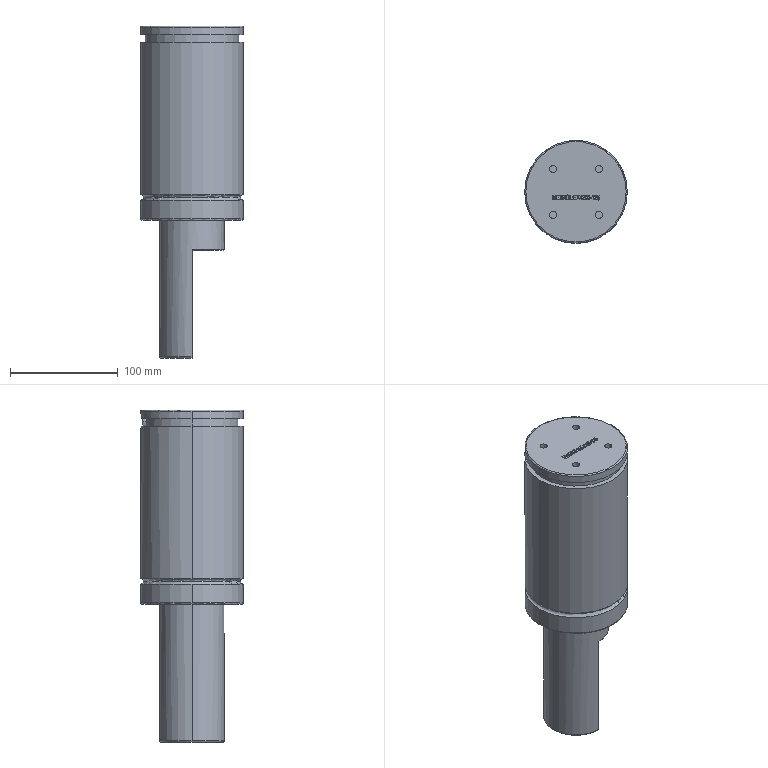Part | STEP file | 1_id2458_x_t | 1 solid | 227 faces | box 95.2 x 95.2 x 308 mm | volume 1486829 mm3 | plane 152 | other 34 | cylinder 27 | cone 8 | torus 6 | commonest cylinder face diameters 6.6 x12 95.2 x6 86.6 x3 14 x2 16.4 x2 60 x2